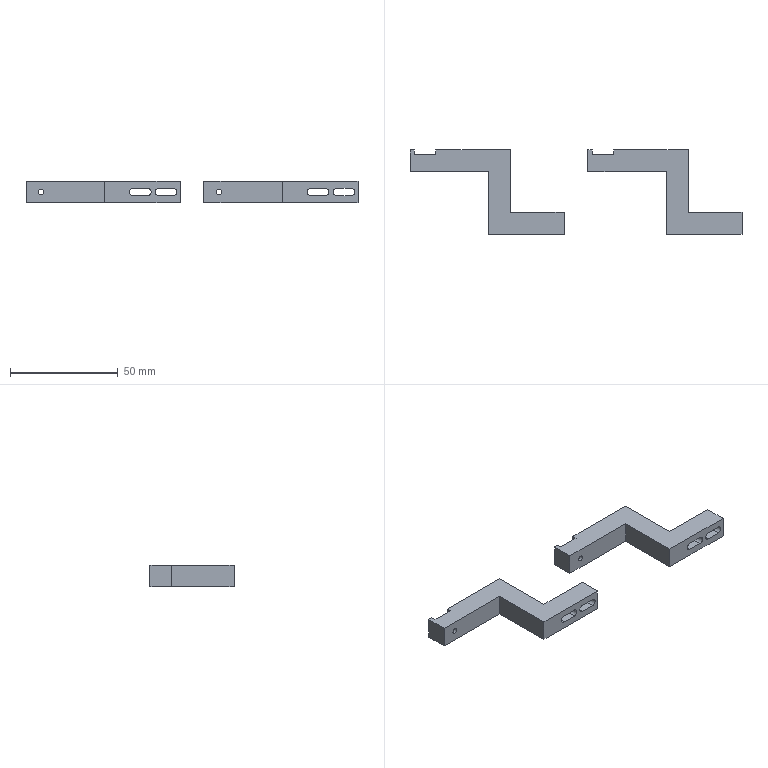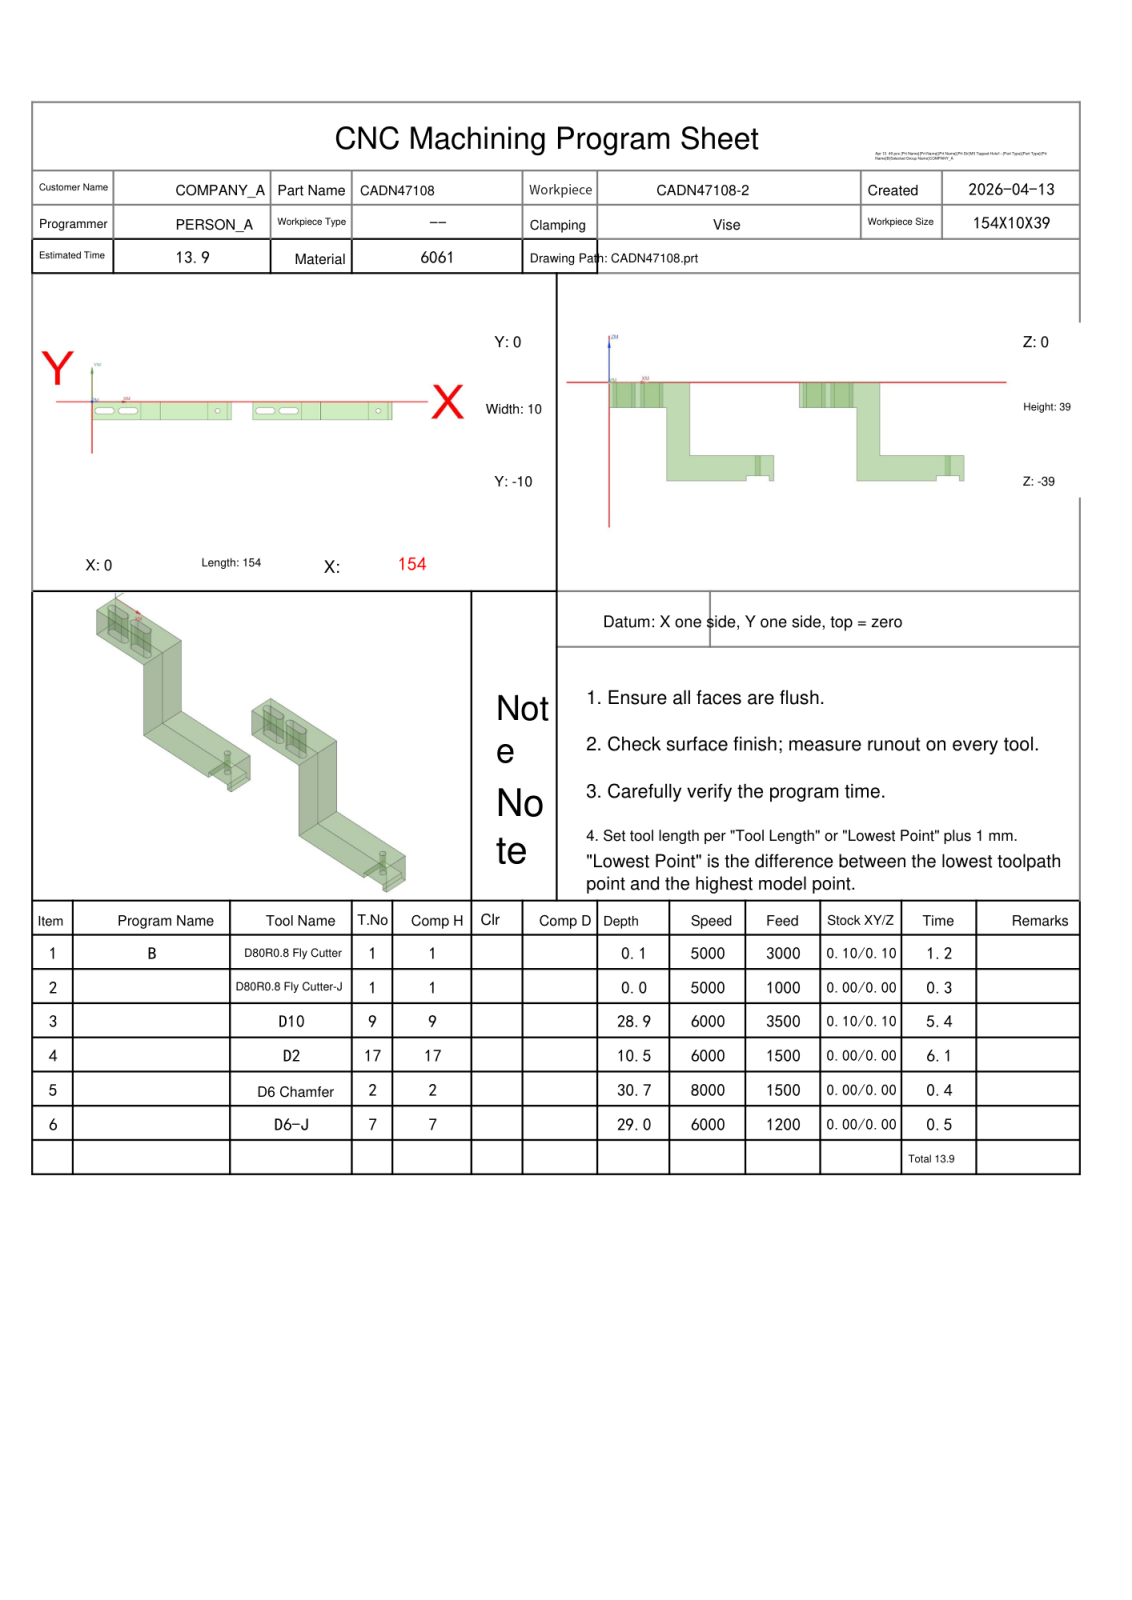NC program | NX | posted by the shop | part box 154 x 39 x 10 mm
Lines 5564 to 5887 of 5887:
N5 T02 M06
(D6 Chamfer  D=6. R=0. H=02 ce=0.00 di=0.00)
G00 G90 G54 X147. Y-5. M03 S8000
G43 H02 Z20.
M08
G98 G81 X147. Y-5. Z-30.75 R-26. F500.
X64.5
G80
G00 Z20.
G00 G90 X99.614 Y1.227 M03 S6500
Z20.
Z.172
G01 Z-1.2 F1500.
G03 X99.9 Y1.027 I1.286 J1.532
G01 X99.946 Y.997
X100. Y1.
X117.5
G02 X118.5 Y0.0 I0.0 J-1.
G01 Y-10.
G02 X117.5 Y-11. I-1. J0.0
G01 X82.5
G02 X81.5 Y-10. I0.0 J1.
G01 Y0.0
G02 X82.5 Y1. I1. J0.0
G01 X100.
X100.054 Y.997
X100.1 Y1.027
G03 X100.386 Y1.227 I-1. J1.732
G01 Z.172
G00 Z2.55
X100.614 Y-5.473
Z.172
G01 Z-1.2
G03 X100.9 Y-5.673 I1.286 J1.532
G01 X100.946 Y-5.703
X101. Y-5.7
X104.3
G03 X105. Y-5. I0.0 J.7
X104.966 Y-4.784 I-.7 J0.0
G01 X104.866 Y-4.589
X104.711 Y-4.434
X104.516 Y-4.334
X104.3 Y-4.3
X97.7
G03 X97. Y-5. I0.0 J-.7
X97.034 Y-5.216 I.7 J0.0
G01 X97.134 Y-5.411
X97.289 Y-5.566
X97.484 Y-5.666
X97.7 Y-5.7
X101.
X101.054 Y-5.703
X101.1 Y-5.673
G03 X101.386 Y-5.473 I-1. J1.732
G01 Z.172
G00 Z10.
X89.386 Y-4.527
Z.172
G01 Z-1.2
G03 X89.1 Y-4.327 I-1.286 J-1.532
G01 X89.054 Y-4.297
X89. Y-4.3
X85.7
G03 X85. Y-5. I0.0 J-.7
X85.034 Y-5.216 I.7 J0.0
G01 X85.134 Y-5.411
X85.289 Y-5.566
X85.484 Y-5.666
X85.7 Y-5.7
X92.3
G03 X93. Y-5. I0.0 J.7
X92.966 Y-4.784 I-.7 J0.0
G01 X92.866 Y-4.589
X92.711 Y-4.434
X92.516 Y-4.334
X92.3 Y-4.3
X89.
X88.946 Y-4.297
X88.9 Y-4.327
G03 X88.614 Y-4.527 I1. J-1.732
G01 Z.172
G00 Z10.
X17.114 Y1.227
Z.172
G01 Z-1.2
G03 X17.4 Y1.027 I1.286 J1.532
G01 X17.446 Y.997
X17.5 Y1.
X35.
G02 X36. Y0.0 I0.0 J-1.
G01 Y-10.
G02 X35. Y-11. I-1. J0.0
G01 X0.0
G02 X-1. Y-10. I0.0 J1.
G01 Y0.0
G02 X0.0 Y1. I1. J0.0
G01 X17.5
X17.554 Y.997
X17.6 Y1.027
G03 X17.886 Y1.227 I-1. J1.732
G01 Z.172
G00 Z2.55
X18.114 Y-5.473
Z.172
G01 Z-1.2
G03 X18.4 Y-5.673 I1.286 J1.532
G01 X18.446 Y-5.703
X18.5 Y-5.7
X21.8
G03 X22.5 Y-5. I0.0 J.7
X22.466 Y-4.784 I-.7 J0.0
G01 X22.366 Y-4.589
X22.211 Y-4.434
X22.016 Y-4.334
X21.8 Y-4.3
X15.2
G03 X14.5 Y-5. I0.0 J-.7
X14.534 Y-5.216 I.7 J0.0
G01 X14.634 Y-5.411
X14.789 Y-5.566
X14.984 Y-5.666
X15.2 Y-5.7
X18.5
X18.554 Y-5.703
X18.6 Y-5.673
G03 X18.886 Y-5.473 I-1. J1.732
G01 Z.172
G00 Z10.
X6.886 Y-4.527
Z.172
G01 Z-1.2
G03 X6.6 Y-4.327 I-1.286 J-1.532
G01 X6.554 Y-4.297
X6.5 Y-4.3
X3.2
G03 X2.5 Y-5. I0.0 J-.7
X2.534 Y-5.216 I.7 J0.0
G01 X2.634 Y-5.411
X2.789 Y-5.566
X2.984 Y-5.666
X3.2 Y-5.7
X9.8
G03 X10.5 Y-5. I0.0 J.7
X10.466 Y-4.784 I-.7 J0.0
G01 X10.366 Y-4.589
X10.211 Y-4.434
X10.016 Y-4.334
X9.8 Y-4.3
X6.5
X6.446 Y-4.297
X6.4 Y-4.327
G03 X6.114 Y-4.527 I1. J-1.732
G01 Z.172
G00 Z10.
X38.021 Y1.068
Z-1.806
G01 Z-30.199
X38.107 Y1.008
X38.137 Y1.
X71.5
G02 X72.5 Y0.0 I0.0 J-1.
G01 Y-10.
G02 X71.5 Y-11. I-1. J0.0
G01 X38.137
X38.107 Y-11.008
X38.021 Y-11.068
Z-1.806
G00 Z10.
X120.521 Y1.068
Z-1.806
G01 Z-30.199
X120.607 Y1.008
X120.637 Y1.
X154.
G02 X155. Y0.0 I0.0 J-1.
G01 Y-10.
G02 X154. Y-11. I-1. J0.0
G01 X120.637
X120.607 Y-11.008
X120.521 Y-11.068
Z-1.806
G00 Z20.
G91 G28 Z0.0
M05
M09
G91 G28 Z0.0
M01
N6 T07 M06
(D6-J  D=6. R=0. H=07 ce=0.30 di=0.00)
G00 G90 G54 X137.7 Y-16. M03 S6000
G43 H07 Z20.
M08
Z-28.5
G01 Z-29. F1200.
Y-10.6
X120.8
Y.6
X154.6
Y-10.6
X137.7
Y-6.4
X125.
Y-3.6
X150.4
Y-6.4
X137.7
X137.2
Y-16.
Z-28.5
G00 Z20.
X55.2 Y6.
Z-28.5
G01 Z-29.
Y.6
X72.1
Y-10.6
X38.3
Y.6
X55.2
Y-3.6
X67.9
Y-6.4
X42.5
Y-3.6
X55.2
X55.7
Y6.
Z-28.5
G00 Z20.
G00 G90 X39.1 Y3.7 M03 S6000
Z20.
Z-6.749
G01 Z-7.249 F1200.
G41 D07
X39.
G03 X38. Y2.7 I0.0 J-1.
G01 Y-12.7
G03 X39. Y-13.7 I1. J0.0
G01 G40 X39.1
Z-6.749
G00 Z20.
Y3.7
Z-13.998
G01 Z-14.498
G41 D07
X39.
G03 X38. Y2.7 I0.0 J-1.
G01 Y-12.7
G03 X39. Y-13.7 I1. J0.0
G01 G40 X39.1
Z-13.998
G00 Z20.
Y3.7
Z-21.246
G01 Z-21.746
G41 D07
X39.
G03 X38. Y2.7 I0.0 J-1.
G01 Y-12.7
G03 X39. Y-13.7 I1. J0.0
G01 G40 X39.1
Z-21.246
G00 Z20.
Y3.7
Z-28.495
G01 Z-28.995
G41 D07
X39.
G03 X38. Y2.7 I0.0 J-1.
G01 Y-12.7
G03 X39. Y-13.7 I1. J0.0
G01 G40 X39.1
Z-28.495
G00 Z20.
X121.6 Y3.7
Z-6.749
G01 Z-7.249
G41 D07
X121.5
G03 X120.5 Y2.7 I0.0 J-1.
G01 Y-12.7
G03 X121.5 Y-13.7 I1. J0.0
G01 G40 X121.6
Z-6.749
G00 Z20.
Y3.7
Z-13.998
G01 Z-14.498
G41 D07
X121.5
G03 X120.5 Y2.7 I0.0 J-1.
G01 Y-12.7
G03 X121.5 Y-13.7 I1. J0.0
G01 G40 X121.6
Z-13.998
G00 Z20.
Y3.7
Z-21.246
G01 Z-21.746
G41 D07
X121.5
G03 X120.5 Y2.7 I0.0 J-1.
G01 Y-12.7
G03 X121.5 Y-13.7 I1. J0.0
G01 G40 X121.6
Z-21.246
G00 Z20.
Y3.7
Z-28.495
G01 Z-28.995
G41 D07
X121.5
G03 X120.5 Y2.7 I0.0 J-1.
G01 Y-12.7
G03 X121.5 Y-13.7 I1. J0.0
G01 G40 X121.6
Z-28.495
G00 Z20.
M05
M09
G91 G28 Z0.0
G91 G28 Y0.0
M30
%